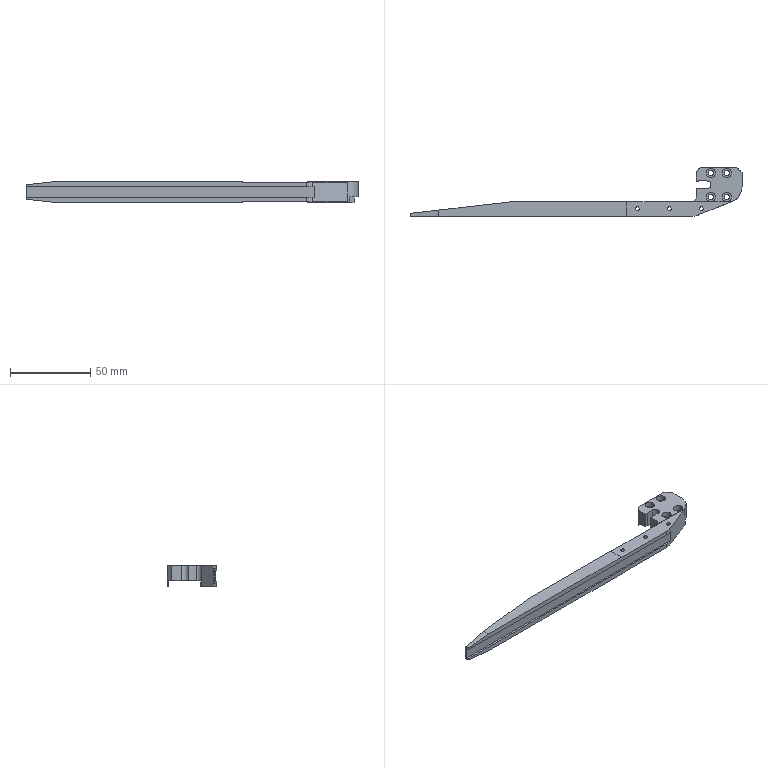NC program | NX | posted by the shop | part box 207.5 x 30.8 x 13 mm
Lines 86 to 1129 of 6162:
N5 T09 M06
(D10  D=10. R=0. H=09 ce=0.10 di=0.10)
G00 G90 G54 X-59. Y29.9 M03 S8000
G43 H09 Z10.2
M08
Z1.
G01 Z-.2 F4000.
Y25.4
G03 X-52. Y18.4 I7. J0.0
G01 X106.25
G02 X106.75 Y17.9 I0.0 J-.5
G01 Y-17.9
G02 X106.25 Y-18.4 I-.5 J0.0
G01 X94.013
G02 X89.053 Y-21.772 I-5.655 J2.985
G01 X88.423 Y-21.839
X87.44 Y-21.9
X-31.75
G02 X-37.516 Y-18.4 I0.0 J6.5
G01 X-106.25
G02 X-106.75 Y-17.9 I0.0 J.5
G01 Y10.936
G02 X-107.75 Y14.4 I5.5 J3.464
X-106.75 Y17.864 I6.5 J0.0
G01 Y17.9
G02 X-106.389 Y18.38 I.5 J0.0
X-105.846 Y18.996 I5.139 J-3.98
G01 X-104.846 Y19.996
G02 X-100.25 Y21.9 I4.596 J-4.596
G01 X-77.646 Y21.899
G02 X-74.946 Y21.264 I-.064 J-6.329
X-73.178 Y20.02 I-2.804 J-5.864
X-72.132 Y18.974 I-9.381 J-10.427
X-71.627 Y18.4 I-4.618 J-4.574
G01 X-50.014
G02 X-49.201 Y17.982 I0.0 J-1.
G01 X-44.799 Y11.818
G03 X-43.986 Y11.4 I.813 J.582
G01 X65.138
G02 X65.928 Y11.012 I-.001 J-1.
G01 X69.76 Y6.052
X69.771 Y6.039
G02 X70.319 Y4.477 I-1.952 J-1.562
X67.819 Y1.977 I-2.5 J0.0
G01 X67.797
X-39.455 Y2.88
G02 X-41.934 Y5.38 I.021 J2.5
X-39.434 Y7.88 I2.5 J0.0
G01 X-39.412
X65.211 Y6.999
X65.219
G03 X65.924 Y7.29 I0.0 J1.
G01 X69.758 Y11.109
G02 X70.464 Y11.4 I.706 J-.709
G01 X98.754
G02 X99.75 Y10.404 I-.004 J-1.
G01 Y-10.404
G02 X98.754 Y-11.4 I-1. J.004
G01 X95.648
G02 X94.666 Y-10.569 I.004 J1.
G03 X91.848 Y-6.298 I-6.221 J-1.04
X88.501 Y-5.12 I-4.175 J-6.517
G01 X87.728 Y-5.015
X72.969 Y-3.319
G02 X72.11 Y-2.552 I.115 J.993
G01 X70.666 Y3.654
G03 X70.457 Y4.071 I-.974 J-.227
G01 X70.41 Y4.2
G02 X70.608 Y4.4 I.2 J0.0
G01 X91.754
G02 X92.75 Y3.404 I-.004 J-1.
G01 Y2.383
G02 X91.75 Y1.387 I-1. J.004
X91.495 Y1.42 I0.0 J1.
G03 X89.363 Y1.827 I-3.822 J-14.236
G01 X88.564 Y1.935
X73.58 Y3.657
X73.466 Y3.664
G03 X72.724 Y3.334 I0.0 J-1.
G01 X67.647 Y-2.286
G02 X66.905 Y-2.615 I-.742 J.671
G01 X66.791 Y-2.608
X40.992 Y.357
G03 X40.25 Y.4 I-.742 J-6.457
G01 X-31.75
G03 X-38.25 Y-6.1 I0.0 J-6.5
G01 Y-9.911
G03 X-37.805 Y-10.615 I.779 J0.0
G01 X-37.45 Y-10.783
X-37.27 Y-10.824
G03 X-36.85 Y-10.404 I0.0 J.42
G01 Y-6.1
G02 X-31.75 Y-1. I5.1 J0.0
G01 X40.25
G02 X40.832 Y-1.033 I0.0 J-5.1
G01 X63.867 Y-3.681
X78.573 Y-5.372
X87.568 Y-6.406
X88.332 Y-6.51
G02 X91.093 Y-7.477 I-.66 J-6.306
X93.353 Y-11.609 I-2.647 J-4.132
G01 Y-15.415
G02 X88.901 Y-20.38 I-4.995 J0.0
G01 X88.332 Y-20.442
X87.44 Y-20.5
X-31.75
G02 X-36.85 Y-15.4 I0.0 J5.1
G01 Y-10.404
G03 X-37.27 Y-9.984 I-.42 J0.0
G01 X-37.45 Y-10.024
X-38.048 Y-10.308
G03 X-38.269 Y-10.592 I.172 J-.361
G02 X-39.246 Y-11.4 I-.981 J.192
G01 X-66.109
G02 X-67.105 Y-10.4 I.004 J1.
X-66.926 Y-9.829 I1. J0.0
G03 X-65.75 Y-6.1 I-5.324 J3.729
X-71.108 Y.299 I-6.5 J0.0
G02 X-71.323 Y.364 I.179 J.984
G03 X-73.908 Y.9 I-2.585 J-5.964
G01 X-98.17
X-98.195
G03 X-98.838 Y.455 I.003 J-.692
G01 X-98.992 Y.053
X-99.02 Y-.097
G03 X-98.6 Y-.517 I.42 J0.0
G01 X-98.567 Y-.515
G02 X-98.17 Y-.5 I.397 J-5.084
G01 X-73.908
G02 X-71.628 Y-1.038 I0.0 J-5.1
X-67.15 Y-6.1 I-.622 J-5.062
X-72.25 Y-11.2 I-5.1 J0.0
G01 X-97.
G02 X-98.894 Y-10.835 I0.0 J5.1
X-99.245 Y-10.695 I2.083 J5.717
G01 X-99.358 Y-10.65
G02 X-100.425 Y-10.174 I5.608 J14.02
X-103.27 Y-5.6 I2.255 J4.574
X-98.567 Y-.515 I5.1 J0.0
G03 X-98.18 Y-.097 I-.033 J.419
X-98.235 Y.112 I-.42 J0.0
G01 X-98.565 Y.686
G03 X-98.865 Y.884 I-.347 J-.199
G02 X-99.75 Y1.874 I.115 J.993
G01 Y6.904
G02 X-98.754 Y7.9 I1. J-.004
G01 X-76.745
G03 X-74.364 Y8.352 I0.0 J6.489
G02 X-73.997 Y8.422 I.367 J-.93
X-73.631 Y8.353 I0.0 J-1.
G01 X-71.837 Y7.648
G03 X-71.471 Y7.579 I.366 J.931
G01 X-71.408 Y7.581
X-64.731 Y8.008
X-64.571 Y8.014
G02 X-62.071 Y5.514 I0.0 J-2.5
X-64.411 Y3.019 I-2.5 J0.0
G01 X-72.12 Y2.525
X-72.28 Y2.52
G02 X-74.78 Y5.02 I0.0 J2.5
X-73.04 Y7.401 I2.5 J0.0
G03 X-72.352 Y8.232 I-.304 J.953
G01 X-72.183 Y9.608
G02 X-72.069 Y9.964 I.993 J-.122
G01 X-71.449 Y11.105
G03 X-71.379 Y11.378 I-.502 J.273
X-71.951 Y11.949 I-.572 J0.0
X-72.434 Y11.682 I0.0 J-.572
G02 X-72.763 Y11.22 I-4.316 J2.718
X-76.745 Y9.3 I-3.982 J3.169
G01 X-101.25
G02 X-106.35 Y14.4 I0.0 J5.1
X-104.856 Y18.006 I5.1 J0.0
G01 X-103.856 Y19.006
G02 X-100.25 Y20.5 I3.606 J-3.606
G01 X-77.665 Y20.499
G02 X-75.554 Y20.003 I-.046 J-4.929
X-74.14 Y19.002 I-2.196 J-4.603
X-73.144 Y18.006 I-8.416 J-9.412
X-71.65 Y14.4 I-3.606 J-3.606
X-72.434 Y11.682 I-5.1 J0.0
G03 X-72.499 Y11.458 I.355 J-.224
X-72.129 Y11.041 I.42 J0.0
G01 X-71.472 Y10.963
X-71.425 Y10.96
G03 X-71.134 Y11.086 I0.0 J.4
G02 X-70.409 Y11.4 I.728 J-.686
G01 X-50.014
G02 X-49.201 Y10.982 I0.0 J-1.
G01 X-44.799 Y4.819
G03 X-43.986 Y4.4 I.814 J.582
G01 X-42.7
G02 X-41.704 Y3.4 I-.004 J-1.
X-41.946 Y2.748 I-1. J0.0
G03 X-45.015 Y-3.59 I10.196 J-8.848
G02 X-45.992 Y-4.4 I-.982 J.19
G01 X-58.008
G02 X-58.985 Y-3.59 I.004 J1.
G03 X-62.054 Y2.748 I-13.265 J-2.51
G02 X-62.296 Y3.4 I.758 J.652
X-61.3 Y4.4 I1. J0.0
G01 X-47.
X-46.5
G03 X-39.5 Y11.4 I0.0 J7.
G01 Y29.9
Z1.
G00 Z3.
G01 X74.181 F6000.
G00 Z.38
G01 Z-.82 F4000.
Y25.4
G03 X81.181 Y18.4 I7. J0.0
G01 X106.25
G02 X106.75 Y17.9 I0.0 J-.5
G01 Y-17.9
G02 X106.25 Y-18.4 I-.5 J0.0
G01 X99.662
G02 X94.394 Y-21.809 I-5.659 J2.971
G01 X92.863 Y-21.9
X-71.824
G02 X-77.952 Y-20.72 I0.0 J16.5
G01 X-83.752 Y-18.4
X-106.25
G02 X-106.75 Y-17.9 I0.0 J.5
G01 Y10.936
G02 X-107.75 Y14.4 I5.5 J3.464
X-106.75 Y17.864 I6.5 J0.0
G01 Y17.9
G02 X-106.389 Y18.38 I.5 J0.0
X-105.846 Y18.996 I5.139 J-3.98
G01 X-104.846 Y19.996
G02 X-100.25 Y21.9 I4.596 J-4.596
G01 X-77.646 Y21.899
G02 X-74.946 Y21.264 I-.064 J-6.329
X-73.178 Y20.02 I-2.804 J-5.864
X-72.132 Y18.974 I-9.381 J-10.427
X-71.627 Y18.4 I-4.618 J-4.574
G01 X86.181
G02 X87.152 Y17.638 I0.0 J-1.
G01 X88.495 Y12.162
G03 X89.465 Y11.4 I.971 J.238
G01 X98.754
G02 X99.75 Y10.404 I-.004 J-1.
G01 Y-6.588
G02 X98.75 Y-7.584 I-1. J.004
X98.109 Y-7.352 I0.0 J1.
G03 X95.162 Y-5.954 I-4.133 J-4.91
G01 X94.048 Y-5.747
X93.836 Y-5.717
X40.992 Y.357
G03 X40.25 Y.4 I-.742 J-6.457
G01 X-71.219
G02 X-71.571 Y.465 I.004 J1.
G03 X-73.908 Y.9 I-2.337 J-6.065
G01 X-98.17
X-98.195
G03 X-98.839 Y.455 I.003 J-.692
G01 X-98.992 Y.053
X-99.02 Y-.097
G03 X-98.6 Y-.517 I.42 J0.0
G01 X-98.567 Y-.515
G02 X-98.17 Y-.5 I.397 J-5.084
G01 X-73.908
G02 X-71.706 Y-1. I0.0 J-5.1
G01 X40.25
G02 X40.832 Y-1.033 I0.0 J-5.1
G01 X63.867 Y-3.681
X65.145 Y-3.828
X78.573 Y-5.372
X81.531 Y-5.712
X93.676 Y-7.108
X93.854 Y-7.133
X94.903 Y-7.33
G02 X98.994 Y-12.262 I-.927 J-4.932
G01 Y-15.429
G02 X94.308 Y-20.411 I-4.992 J0.0
G01 X92.863 Y-20.5
X-71.824
G02 X-77.432 Y-19.42 I0.0 J15.1
G01 X-98.894 Y-10.835
G02 X-99.245 Y-10.695 I2.083 J5.717
G01 X-99.357 Y-10.65
G02 X-100.425 Y-10.174 I5.607 J14.02
X-103.27 Y-5.6 I2.255 J4.574
X-98.567 Y-.515 I5.1 J0.0
G03 X-98.18 Y-.097 I-.033 J.419
X-98.236 Y.112 I-.42 J0.0
G01 X-98.565 Y.686
G03 X-98.865 Y.884 I-.347 J-.199
G02 X-99.75 Y1.874 I.115 J.993
G01 Y6.904
G02 X-98.754 Y7.9 I1. J-.004
G01 X-76.745
G03 X-74.512 Y8.296 I0.0 J6.489
G02 X-74.217 Y8.349 I.295 J-.804
X-73.932 Y8.3 I0.0 J-.856
G01 X-72.879 Y7.928
G03 X-72.547 Y7.871 I.332 J.943
G01 X-72.389 Y7.884
G02 X-71.99 Y7.916 I.399 J-2.468
G01 X-71.973
X67.835 Y6.981
G02 X70.319 Y4.481 I-.017 J-2.5
X67.819 Y1.981 I-2.5 J0.0
G01 X67.802
X-72.006 Y2.916
G02 X-74.49 Y5.416 I.017 J2.5
X-73.396 Y7.483 I2.5 J0.0
G03 X-73.035 Y7.926 I-.563 J.826
G01 X-72.355 Y9.569
X-72.292 Y9.695
X-71.467 Y11.092
G03 X-71.388 Y11.38 I-.488 J.288
X-71.955 Y11.947 I-.567 J0.0
X-72.434 Y11.682 I0.0 J-.567
G02 X-72.763 Y11.22 I-4.316 J2.718
X-76.745 Y9.3 I-3.982 J3.169
G01 X-76.75
X-101.25
G02 X-106.35 Y14.4 I0.0 J5.1
X-104.856 Y18.006 I5.1 J0.0
G01 X-103.856 Y19.006
G02 X-100.25 Y20.5 I3.606 J-3.606
G01 X-77.665 Y20.499
G02 X-75.554 Y20.003 I-.046 J-4.929
X-74.14 Y19.002 I-2.196 J-4.603
X-73.144 Y18.006 I-8.416 J-9.412
X-71.65 Y14.4 I-3.606 J-3.606
X-72.434 Y11.682 I-5.1 J0.0
G03 X-72.499 Y11.459 I.355 J-.224
X-72.129 Y11.041 I.42 J0.0
G01 X-71.472 Y10.963
X-71.425 Y10.96
G03 X-71.134 Y11.085 I0.0 J.4
G02 X-70.409 Y11.4 I.728 J-.685
G01 X83.167
G02 X83.98 Y10.982 I-.001 J-1.
G01 X88.382 Y4.819
G03 X89.196 Y4.4 I.814 J.581
G01 X91.754
G02 X92.75 Y3.404 I-.004 J-1.
G01 Y2.571
G02 X91.75 Y1.575 I-1. J.004
G01 X91.64 Y1.581
X70.585 Y4.002
G02 X70.41 Y4.2 I.025 J.198
X70.608 Y4.4 I.2 J0.0
G01 X86.181
X86.681
G03 X93.681 Y11.4 I0.0 J7.
G01 Y29.9
Z.38
G00 Z2.8
G01 X74.181 F6000.
G00 Z-.24
G01 Z-1.44 F4000.
Y25.4
G03 X81.181 Y18.4 I7. J0.0
G01 X106.25
G02 X106.75 Y17.9 I0.0 J-.5
G01 Y-17.9
G02 X106.25 Y-18.4 I-.5 J0.0
G01 X105.201
G02 X100.684 Y-21.704 I-5.659 J2.998
X98.486 Y-21.901 I-2.198 J12.128
G01 X98.318 Y-21.9
X-71.824
G02 X-77.952 Y-20.72 I0.0 J16.5
G01 X-83.752 Y-18.4
X-106.25
G02 X-106.75 Y-17.9 I0.0 J.5
G01 Y10.936
G02 X-107.75 Y14.4 I5.5 J3.464
X-106.75 Y17.864 I6.5 J0.0
G01 Y17.9
G02 X-106.389 Y18.38 I.5 J0.0
X-105.846 Y18.996 I5.139 J-3.98
G01 X-104.846 Y19.996
G02 X-100.25 Y21.9 I4.596 J-4.596
G01 X-77.646 Y21.899
G02 X-74.946 Y21.264 I-.064 J-6.329
X-73.178 Y20.02 I-2.804 J-5.864
X-72.132 Y18.974 I-9.381 J-10.427
X-71.627 Y18.4 I-4.618 J-4.574
G01 X86.181
G02 X87.153 Y17.638 I0.0 J-1.
G01 X88.495 Y12.162
G03 X89.465 Y11.4 I.971 J.238
G01 X98.754
G02 X99.75 Y10.404 I-.004 J-1.
G01 Y-5.28
G02 X98.75 Y-6.276 I-1. J.004
G01 X98.64 Y-6.27
X40.992 Y.357
G03 X40.25 Y.4 I-.742 J-6.457
G01 X-71.22
G02 X-71.571 Y.465 I.004 J1.
G03 X-73.908 Y.9 I-2.337 J-6.065
G01 X-98.17
X-98.195
G03 X-98.839 Y.455 I.003 J-.692
G01 X-98.992 Y.053
X-99.02 Y-.097
G03 X-98.6 Y-.517 I.42 J0.0
G01 X-98.567 Y-.515
G02 X-98.17 Y-.5 I.397 J-5.084
G01 X-73.908
G02 X-71.706 Y-1. I0.0 J-5.1
G01 X40.25
G02 X40.832 Y-1.033 I0.0 J-5.1
G01 X78.573 Y-5.372
X81.531 Y-5.712
X93.676 Y-7.108
X99.142 Y-7.737
X100.347 Y-7.941
G02 X104.547 Y-12.913 I-.843 J-4.972
G01 Y-15.402
G02 X100.435 Y-20.326 I-5.004 J0.0
X98.486 Y-20.501 I-1.949 J10.751
G01 X98.327 Y-20.5
X-71.824
G02 X-77.432 Y-19.42 I0.0 J15.1
G01 X-98.894 Y-10.835
G02 X-99.245 Y-10.695 I2.083 J5.717
G01 X-99.356 Y-10.65
G02 X-100.427 Y-10.173 I5.606 J14.021
X-103.27 Y-5.6 I2.257 J4.573
X-98.567 Y-.515 I5.1 J0.0
G03 X-98.18 Y-.097 I-.033 J.419
X-98.236 Y.112 I-.42 J0.0
G01 X-98.565 Y.686
G03 X-98.866 Y.884 I-.347 J-.199
G02 X-99.75 Y1.873 I.115 J.993
G01 Y6.904
G02 X-98.754 Y7.9 I1. J-.004
G01 X-76.745
G03 X-74.512 Y8.296 I0.0 J6.489
G02 X-74.217 Y8.349 I.295 J-.804
X-73.932 Y8.3 I0.0 J-.856
G01 X-72.879 Y7.928
G03 X-72.547 Y7.871 I.332 J.943
G01 X-72.389 Y7.884
G02 X-71.99 Y7.916 I.399 J-2.468
G01 X-71.973
X67.835 Y6.981
G02 X70.319 Y4.481 I-.017 J-2.5
X67.819 Y1.981 I-2.5 J0.0
G01 X67.802
X-72.006 Y2.916
G02 X-74.49 Y5.416 I.017 J2.5
X-73.396 Y7.483 I2.5 J0.0
G03 X-73.035 Y7.926 I-.563 J.826
G01 X-72.355 Y9.57
X-72.292 Y9.696
X-71.467 Y11.092
G03 X-71.388 Y11.38 I-.488 J.288
X-71.955 Y11.947 I-.567 J0.0
X-72.434 Y11.682 I0.0 J-.567
G02 X-72.763 Y11.22 I-4.316 J2.718
X-76.745 Y9.3 I-3.982 J3.169
G01 X-76.75
X-101.25
G02 X-106.35 Y14.4 I0.0 J5.1
X-104.856 Y18.006 I5.1 J0.0
G01 X-103.856 Y19.006
G02 X-100.25 Y20.5 I3.606 J-3.606
G01 X-77.665 Y20.499
G02 X-75.554 Y20.003 I-.046 J-4.929
X-74.14 Y19.002 I-2.196 J-4.603
X-73.144 Y18.006 I-8.416 J-9.412
X-71.65 Y14.4 I-3.606 J-3.606
X-72.434 Y11.682 I-5.1 J0.0
G03 X-72.499 Y11.459 I.355 J-.224
X-72.129 Y11.042 I.42 J0.0
G01 X-71.471 Y10.963
X-71.424 Y10.96
G03 X-71.134 Y11.086 I0.0 J.4
G02 X-70.41 Y11.4 I.728 J-.686
G01 X83.168
G02 X83.98 Y10.982 I-.001 J-1.
G01 X88.382 Y4.819
G03 X89.196 Y4.4 I.814 J.581
G01 X91.755
G02 X92.75 Y3.405 I-.004 J-1.
G01 Y2.571
G02 X91.75 Y1.575 I-1. J.004
G01 X91.64 Y1.581
X70.585 Y4.002
G02 X70.41 Y4.2 I.025 J.198
X70.608 Y4.4 I.2 J0.0
G01 X86.181
X86.681
G03 X93.681 Y11.4 I0.0 J7.
G01 Y29.9
Z-.24
G00 Z2.18
G01 X74.181 F6000.
G00 Z-.86
G01 Z-2.06 F4000.
Y25.4
G03 X81.181 Y18.4 I7. J0.0
G01 X106.25
G02 X106.75 Y17.9 I0.0 J-.5
G01 Y-7.784
G02 X110.25 Y-13.846 I-3.5 J-6.062
G01 Y-14.4
G02 X102.75 Y-21.9 I-7.5 J0.0
G01 X-71.824
G02 X-77.952 Y-20.72 I0.0 J16.5
G01 X-83.752 Y-18.4
X-106.25
G02 X-106.75 Y-17.9 I0.0 J.5
G01 Y10.936
G02 X-107.75 Y14.4 I5.5 J3.464
X-106.75 Y17.864 I6.5 J0.0
G01 Y17.9
G02 X-106.389 Y18.38 I.5 J0.0
X-105.846 Y18.996 I5.139 J-3.98
G01 X-104.846 Y19.996
G02 X-100.25 Y21.9 I4.596 J-4.596
G01 X-77.646 Y21.899
G02 X-74.946 Y21.264 I-.064 J-6.329
X-73.178 Y20.02 I-2.804 J-5.864
X-72.132 Y18.974 I-9.381 J-10.427
X-71.627 Y18.4 I-4.618 J-4.574
G01 X86.181
G02 X87.153 Y17.638 I0.0 J-1.
G01 X88.495 Y12.162
G03 X89.466 Y11.4 I.971 J.238
G01 X98.754
G02 X99.75 Y10.404 I-.004 J-1.
G01 Y-5.28
G02 X98.75 Y-6.276 I-1. J.004
G01 X98.64 Y-6.27
X40.992 Y.357
G03 X40.25 Y.4 I-.742 J-6.457
G01 X-71.22
G02 X-71.571 Y.465 I.004 J1.
G03 X-73.908 Y.9 I-2.337 J-6.065
G01 X-98.171
X-98.195
G03 X-98.839 Y.455 I.003 J-.692
G01 X-98.993 Y.053
X-99.02 Y-.097
G03 X-98.6 Y-.517 I.42 J0.0
G01 X-98.568 Y-.516
G02 X-98.17 Y-.5 I.398 J-5.084
G01 X-98.16
X-73.908
G02 X-71.706 Y-1. I0.0 J-5.1
G01 X40.25
G02 X40.832 Y-1.033 I0.0 J-5.1
G01 X81.09 Y-5.661
X81.531 Y-5.712
X83.818 Y-5.975
X103.89 Y-8.282
G02 X108.85 Y-13.846 I-.64 J-5.563
G01 Y-14.4
G02 X102.75 Y-20.5 I-6.1 J0.0
G01 X-71.824
G02 X-77.432 Y-19.42 I0.0 J15.1
G01 X-98.894 Y-10.835
G02 X-99.245 Y-10.695 I2.083 J5.717
G01 X-99.355 Y-10.651
G02 X-100.428 Y-10.173 I5.605 J14.021
X-103.27 Y-5.6 I2.258 J4.573
X-98.568 Y-.516 I5.1 J0.0
G03 X-98.18 Y-.097 I-.033 J.419
X-98.236 Y.112 I-.42 J0.0
G01 X-98.565 Y.686
G03 X-98.866 Y.884 I-.347 J-.199
G02 X-99.75 Y1.873 I.116 J.993
G01 Y6.904
G02 X-98.754 Y7.9 I1. J-.004
G01 X-76.745
G03 X-74.512 Y8.296 I0.0 J6.489
G02 X-74.217 Y8.349 I.295 J-.804
X-73.932 Y8.3 I0.0 J-.856
G01 X-72.879 Y7.928
G03 X-72.547 Y7.871 I.332 J.943
G01 X-72.389 Y7.884
G02 X-71.99 Y7.916 I.399 J-2.468
G01 X-71.973
X67.835 Y6.981
G02 X70.318 Y4.481 I-.017 J-2.5
X67.818 Y1.981 I-2.5 J0.0
G01 X67.802
X-72.006 Y2.916
G02 X-74.49 Y5.416 I.017 J2.5
X-73.396 Y7.483 I2.5 J0.0
G03 X-73.035 Y7.926 I-.563 J.826
G01 X-72.355 Y9.57
X-72.292 Y9.696
X-71.467 Y11.092
G03 X-71.388 Y11.381 I-.488 J.288
X-71.955 Y11.948 I-.567 J0.0
X-72.434 Y11.683 I0.0 J-.567
G02 X-72.763 Y11.22 I-4.316 J2.717
X-76.745 Y9.3 I-3.982 J3.169
G01 X-76.75
X-101.25
G02 X-106.35 Y14.4 I0.0 J5.1
X-104.856 Y18.006 I5.1 J0.0
G01 X-103.856 Y19.006
G02 X-100.25 Y20.5 I3.606 J-3.606
G01 X-77.665 Y20.499
G02 X-75.554 Y20.003 I-.046 J-4.929
X-74.14 Y19.002 I-2.196 J-4.603
X-73.144 Y18.006 I-8.416 J-9.412
X-71.65 Y14.4 I-3.606 J-3.606
X-72.434 Y11.683 I-5.1 J0.0
G03 X-72.499 Y11.459 I.355 J-.224
X-72.129 Y11.042 I.42 J0.0
G01 X-71.471 Y10.963
X-71.424 Y10.961
G03 X-71.134 Y11.086 I0.0 J.4
G02 X-70.41 Y11.4 I.728 J-.686
G01 X83.168
G02 X83.98 Y10.982 I-.001 J-1.
G01 X88.382 Y4.819
G03 X89.196 Y4.4 I.814 J.581
G01 X91.755
G02 X92.75 Y3.405 I-.005 J-1.
G01 Y2.57
G02 X91.75 Y1.575 I-1. J.005
G01 X91.641 Y1.581
X70.585 Y4.002
G02 X70.41 Y4.2 I.025 J.198
X70.608 Y4.4 I.2 J0.0
G01 X86.181
X86.681
G03 X93.681 Y11.4 I0.0 J7.
G01 Y29.9
Z-.86
G00 Z1.56
G01 X74.181 F6000.
G00 Z-1.48
G01 Z-2.68 F4000.
Y25.4
G03 X81.181 Y18.4 I7. J0.0
G01 X106.25
G02 X106.75 Y17.9 I0.0 J-.5
G01 Y-7.784
G02 X110.25 Y-13.846 I-3.5 J-6.062
G01 Y-14.4
G02 X102.75 Y-21.9 I-7.5 J0.0
G01 X-71.824
G02 X-77.952 Y-20.72 I0.0 J16.5
G01 X-83.752 Y-18.4
X-106.25
G02 X-106.75 Y-17.9 I0.0 J.5
G01 Y10.936
G02 X-107.75 Y14.4 I5.5 J3.464
X-106.75 Y17.864 I6.5 J0.0
G01 Y17.9
G02 X-106.389 Y18.38 I.5 J0.0
X-105.846 Y18.996 I5.139 J-3.98
G01 X-104.846 Y19.996
G02 X-100.25 Y21.9 I4.596 J-4.596
G01 X-77.646 Y21.899
G02 X-74.946 Y21.264 I-.064 J-6.329
X-73.178 Y20.02 I-2.804 J-5.864
X-72.132 Y18.974 I-9.381 J-10.427
X-71.627 Y18.4 I-4.618 J-4.574
G01 X86.181
G02 X87.153 Y17.638 I0.0 J-1.
G01 X88.495 Y12.162
G03 X89.466 Y11.4 I.971 J.238
G01 X98.755
G02 X99.75 Y10.405 I-.005 J-1.
G01 Y-5.28
G02 X98.75 Y-6.276 I-1. J.005
G01 X98.64 Y-6.27
X40.992 Y.357
G03 X40.25 Y.4 I-.742 J-6.457
G01 X-71.22
G02 X-71.571 Y.465 I.005 J1.
G03 X-73.908 Y.9 I-2.338 J-6.065
G01 X-98.173
X-98.196
G03 X-98.839 Y.455 I.003 J-.692
G01 X-98.993 Y.053
X-99.02 Y-.097
G03 X-98.6 Y-.517 I.42 J0.0
G01 X-98.568 Y-.516
G02 X-98.17 Y-.5 I.398 J-5.084
G01 X-98.16
X-73.908
G02 X-71.706 Y-1. I0.0 J-5.1
G01 X40.25
G02 X40.832 Y-1.033 I0.0 J-5.1
G01 X103.89 Y-8.282
G02 X108.85 Y-13.846 I-.64 J-5.563
G01 Y-14.4
G02 X102.75 Y-20.5 I-6.1 J0.0
G01 X-71.824
G02 X-77.432 Y-19.42 I0.0 J15.1
G01 X-98.894 Y-10.835
G02 X-99.245 Y-10.695 I2.083 J5.717
G01 X-99.355 Y-10.651
G02 X-100.43 Y-10.172 I5.605 J14.021
X-103.27 Y-5.6 I2.26 J4.572
X-98.568 Y-.516 I5.1 J0.0
G03 X-98.18 Y-.097 I-.033 J.419
X-98.236 Y.112 I-.42 J0.0
G01 X-98.566 Y.686
G03 X-98.866 Y.884 I-.347 J-.199
G02 X-99.75 Y1.873 I.116 J.993
G01 Y6.905
G02 X-98.755 Y7.9 I1. J-.005
G01 X-76.745
G03 X-74.512 Y8.296 I0.0 J6.489
G02 X-74.217 Y8.349 I.295 J-.804
X-73.932 Y8.3 I0.0 J-.856
G01 X-72.879 Y7.928
G03 X-72.547 Y7.871 I.332 J.943
G01 X-72.389 Y7.884
G02 X-71.99 Y7.916 I.399 J-2.468
G01 X-71.973
X67.835 Y6.981
G02 X70.318 Y4.481 I-.017 J-2.5
X67.818 Y1.981 I-2.5 J0.0
G01 X67.802
X-72.006 Y2.916
G02 X-74.49 Y5.416 I.017 J2.5
X-73.396 Y7.483 I2.5 J0.0
G03 X-73.035 Y7.926 I-.563 J.826
G01 X-72.355 Y9.57
X-72.292 Y9.696
X-71.467 Y11.092
G03 X-71.388 Y11.381 I-.488 J.288
X-71.954 Y11.948 I-.567 J0.0
X-72.434 Y11.683 I0.0 J-.567
G02 X-72.763 Y11.22 I-4.316 J2.717
X-76.745 Y9.3 I-3.982 J3.169
G01 X-76.75
X-101.25
G02 X-106.35 Y14.4 I0.0 J5.1
X-104.856 Y18.006 I5.1 J0.0
G01 X-103.856 Y19.006
G02 X-100.25 Y20.5 I3.606 J-3.606
G01 X-77.664 Y20.499
G02 X-75.554 Y20.003 I-.046 J-4.929
X-74.14 Y19.002 I-2.196 J-4.603
X-73.144 Y18.006 I-8.416 J-9.412
X-71.65 Y14.4 I-3.606 J-3.606
X-72.434 Y11.683 I-5.1 J0.0
G03 X-72.499 Y11.459 I.355 J-.224
X-72.129 Y11.042 I.42 J0.0
G01 X-71.471 Y10.963
X-71.424 Y10.961
G03 X-71.133 Y11.086 I0.0 J.4
G02 X-70.41 Y11.4 I.728 J-.686
G01 X83.168
G02 X83.98 Y10.982 I-.001 J-1.
G01 X88.382 Y4.819
G03 X89.196 Y4.4 I.814 J.581
G01 X91.755
G02 X92.75 Y3.405 I-.005 J-1.
G01 Y2.57
G02 X91.75 Y1.575 I-1. J.005
G01 X91.641 Y1.581
X70.585 Y4.002
G02 X70.41 Y4.2 I.025 J.198
X70.608 Y4.4 I.2 J0.0
G01 X86.181
X86.681
G03 X93.681 Y11.4 I0.0 J7.
G01 Y29.9
Z-1.48
G00 Z.94
G01 X74.181 F6000.
G00 Z-2.1
G01 Z-3.3 F4000.
Y25.4
G03 X81.181 Y18.4 I7. J0.0
G01 X106.25
G02 X106.75 Y17.9 I0.0 J-.5
G01 Y-7.784
G02 X110.25 Y-13.846 I-3.5 J-6.062
G01 Y-14.4
G02 X102.75 Y-21.9 I-7.5 J0.0
G01 X-71.824
G02 X-77.952 Y-20.72 I0.0 J16.5
G01 X-83.752 Y-18.4
X-106.25
G02 X-106.75 Y-17.9 I0.0 J.5
G01 Y10.936
G02 X-107.75 Y14.4 I5.5 J3.464
X-106.75 Y17.864 I6.5 J0.0
G01 Y17.9
G02 X-106.389 Y18.38 I.5 J0.0
X-105.846 Y18.996 I5.139 J-3.98
G01 X-104.846 Y19.996
G02 X-100.25 Y21.9 I4.596 J-4.596
G01 X-77.646 Y21.899
G02 X-74.946 Y21.264 I-.064 J-6.329
X-73.178 Y20.02 I-2.804 J-5.864
X-72.132 Y18.974 I-9.381 J-10.427
X-71.627 Y18.4 I-4.618 J-4.574
G01 X86.181
G02 X87.153 Y17.638 I0.0 J-1.
G01 X88.495 Y12.162
G03 X89.466 Y11.4 I.971 J.238
G01 X98.755
G02 X99.75 Y10.405 I-.005 J-1.
G01 Y-5.281
G02 X98.75 Y-6.276 I-1. J.005
G01 X98.641 Y-6.27
X40.992 Y.357
G03 X40.25 Y.4 I-.742 J-6.457
G01 X-71.22
G02 X-71.571 Y.465 I.005 J1.
G03 X-73.908 Y.9 I-2.338 J-6.065
G01 X-98.175
X-98.196
G03 X-98.84 Y.455 I.003 J-.692
G01 X-98.993 Y.053
X-99.021 Y-.097
G03 X-98.601 Y-.517 I.42 J0.0
G01 X-98.568 Y-.516
G02 X-98.17 Y-.5 I.398 J-5.084
G01 X-98.16
X-73.908
G02 X-71.706 Y-1. I0.0 J-5.1
G01 X40.25
G02 X40.832 Y-1.033 I0.0 J-5.1
G01 X103.89 Y-8.282
G02 X108.85 Y-13.846 I-.64 J-5.563
G01 Y-14.4
G02 X102.75 Y-20.5 I-6.1 J0.0
G01 X-71.824
G02 X-77.432 Y-19.42 I0.0 J15.1
G01 X-98.894 Y-10.835
G02 X-99.245 Y-10.695 I2.083 J5.717
G01 X-99.354 Y-10.651
G02 X-100.432 Y-10.171 I5.604 J14.021
X-103.27 Y-5.6 I2.261 J4.571
X-98.568 Y-.516 I5.1 J0.0
G03 X-98.181 Y-.097 I-.033 J.419
X-98.236 Y.112 I-.42 J0.0
G01 X-98.566 Y.686
G03 X-98.866 Y.884 I-.347 J-.199
G02 X-99.75 Y1.873 I.116 J.993
G01 Y6.905
G02 X-98.755 Y7.9 I1. J-.005
G01 X-76.745
G03 X-74.512 Y8.296 I0.0 J6.489
G02 X-74.217 Y8.349 I.295 J-.804
X-73.932 Y8.3 I0.0 J-.856
G01 X-72.879 Y7.928
G03 X-72.547 Y7.871 I.332 J.943
G01 X-72.389 Y7.884
G02 X-71.99 Y7.916 I.399 J-2.468
G01 X-71.973
X67.835 Y6.981
G02 X70.318 Y4.481 I-.017 J-2.5
X67.818 Y1.981 I-2.5 J0.0
G01 X67.802
X-72.006 Y2.916
G02 X-74.49 Y5.416 I.017 J2.5
X-73.396 Y7.483 I2.5 J0.0
G03 X-73.035 Y7.926 I-.563 J.826
G01 X-72.355 Y9.57
X-72.292 Y9.696
X-71.467 Y11.093
G03 X-71.388 Y11.381 I-.488 J.288
X-71.954 Y11.948 I-.567 J0.0
X-72.434 Y11.683 I0.0 J-.567
G02 X-72.763 Y11.22 I-4.316 J2.717
X-76.745 Y9.3 I-3.982 J3.169
G01 X-76.75
X-101.25
G02 X-106.35 Y14.4 I0.0 J5.1
X-104.856 Y18.006 I5.1 J0.0
G01 X-103.856 Y19.006
G02 X-100.25 Y20.5 I3.606 J-3.606
G01 X-77.664 Y20.499
G02 X-75.554 Y20.003 I-.046 J-4.929
X-74.14 Y19.002 I-2.196 J-4.603
X-73.144 Y18.006 I-8.416 J-9.412
X-71.65 Y14.4 I-3.606 J-3.606
X-72.434 Y11.683 I-5.1 J0.0
G03 X-72.499 Y11.459 I.355 J-.224
X-72.128 Y11.042 I.42 J0.0
G01 X-71.471 Y10.964
X-71.424 Y10.961
G03 X-71.133 Y11.086 I0.0 J.4
G02 X-70.41 Y11.4 I.728 J-.686
G01 X83.168
G02 X83.98 Y10.982 I-.001 J-1.
G01 X88.382 Y4.819
G03 X89.196 Y4.4 I.814 J.581
G01 X91.755
G02 X92.75 Y3.405 I-.005 J-1.
G01 Y2.57
G02 X91.75 Y1.575 I-1. J.005
G01 X91.641 Y1.581
X70.585 Y4.002
G02 X70.41 Y4.2 I.025 J.198
X70.608 Y4.4 I.2 J0.0
G01 X86.181
X86.681
G03 X93.681 Y11.4 I0.0 J7.
G01 Y29.9
Z-2.1
G00 Z.32
G01 X74.181 F6000.
G00 Z-2.59
G01 Z-3.79 F4000.
Y25.4
G03 X81.181 Y18.4 I7. J0.0
G01 X106.25
G02 X106.75 Y17.9 I0.0 J-.5
G01 Y-7.784
G02 X110.25 Y-13.846 I-3.5 J-6.062
G01 Y-14.4
G02 X102.75 Y-21.9 I-7.5 J0.0
G01 X-71.824
G02 X-77.952 Y-20.72 I0.0 J16.5
G01 X-83.752 Y-18.4
X-106.25
G02 X-106.75 Y-17.9 I0.0 J.5
G01 Y-6.791
G02 X-110.25 Y3.37 I13. J10.161
G01 Y11.9
G02 X-108.346 Y16.496 I6.5 J0.0
G01 X-106.668 Y18.174
G02 X-106.524 Y18.318 I.418 J-.274
G01 X-104.846 Y19.996
G02 X-100.25 Y21.9 I4.596 J-4.596
G01 X-77.646 Y21.899
G02 X-74.946 Y21.264 I-.064 J-6.329
X-73.178 Y20.02 I-2.804 J-5.864
X-72.133 Y18.975 I-9.381 J-10.427
G01 X-71.558 Y18.4
X86.181
G02 X87.153 Y17.638 I0.0 J-1.
G01 X88.495 Y12.162
G03 X89.466 Y11.4 I.971 J.238
G01 X98.755
G02 X99.75 Y10.405 I-.005 J-1.
G01 Y-5.281
G02 X98.75 Y-6.276 I-1. J.005
G01 X98.641 Y-6.27
X40.992 Y.357
G03 X40.25 Y.4 I-.742 J-6.457
G01 X-67.755
G02 X-68.75 Y1.395 I.005 J1.
G01 Y2.15
G03 X-69.051 Y4.104 I-6.5 J0.0
G02 X-69.095 Y4.4 I.955 J.296
X-69.051 Y4.696 I1. J0.0
G03 X-68.823 Y5.68 I-6.199 J1.954
G01 X-68.791 Y5.734
X-68.728 Y5.781
X-68.661 Y5.796
X-68.678 Y5.862
G02 X-66.218 Y7.917 I2.46 J-.445
G01 X-66.201
X67.836 Y6.981
G02 X70.318 Y4.481 I-.017 J-2.5
X67.818 Y1.981 I-2.5 J0.0
G01 X67.801
X-66.236 Y2.917
G02 X-68.718 Y5.417 I.017 J2.5
X-68.706 Y5.666 I2.5 J0.0
G01 X-68.722 Y5.724
X-68.77 Y5.785
X-68.83 Y5.82
X-68.796 Y5.881
G03 X-68.75 Y6.65 I-6.454 J.769
G01 Y9.913
G03 X-69.195 Y10.616 I-.779 J0.0
G01 X-69.55 Y10.784
X-69.73 Y10.825
G03 X-70.15 Y10.405 I0.0 J-.42
G01 Y6.65
G02 X-70.673 Y4.4 I-5.1 J0.0
X-70.15 Y2.15 I-4.577 J-2.25
G01 Y-1.
X40.25
G02 X40.832 Y-1.033 I0.0 J-5.1
G01 X103.89 Y-8.282
G02 X108.85 Y-13.846 I-.64 J-5.563
G01 Y-14.4
G02 X102.75 Y-20.5 I-6.1 J0.0
G01 X-71.824
G02 X-77.432 Y-19.42 I0.0 J15.1
G01 X-98.894 Y-10.835
G02 X-99.245 Y-10.695 I2.083 J5.717
G01 X-99.354 Y-10.651
G02 X-108.85 Y3.37 I5.604 J14.022
G01 Y11.9
G02 X-107.356 Y15.506 I5.1 J0.0
G01 X-103.856 Y19.006
G02 X-100.25 Y20.5 I3.606 J-3.606
G01 X-77.664 Y20.499
G02 X-75.554 Y20.003 I-.046 J-4.929
X-74.14 Y19.002 I-2.196 J-4.603
X-73.15 Y18.012 I-8.419 J-9.409
G01 X-71.644 Y16.506
G02 X-70.15 Y12.9 I-3.606 J-3.606
G01 Y10.405
G03 X-69.73 Y9.985 I.42 J0.0
G01 X-69.55 Y10.026
X-68.952 Y10.309
G03 X-68.731 Y10.593 I-.172 J.361
G02 X-67.755 Y11.4 I.981 J-.193
G01 X83.168
G02 X83.98 Y10.982 I-.001 J-1.
G01 X88.383 Y4.819
G03 X89.196 Y4.4 I.814 J.581
G01 X91.755
G02 X92.75 Y3.405 I-.005 J-1.
G01 Y2.57
G02 X91.75 Y1.575 I-1. J.005
G01 X91.641 Y1.581
X70.585 Y4.002
G02 X70.41 Y4.2 I.025 J.198
X70.608 Y4.4 I.2 J0.0
G01 X86.181
X86.681
G03 X93.681 Y11.4 I0.0 J7.
G01 Y29.9
Z-2.59
G00 Z-.3
G01 X74.182 F6000.
G00 Z-3.08
G01 Z-4.28 F4000.
Y25.4
G03 X81.182 Y18.4 I7. J0.0
G01 X106.25
G02 X106.75 Y17.9 I0.0 J-.5
G01 Y-7.784
G02 X110.25 Y-13.846 I-3.5 J-6.062
G01 Y-14.4
G02 X102.75 Y-21.9 I-7.5 J0.0
G01 X-71.824
G02 X-77.952 Y-20.72 I0.0 J16.5
G01 X-83.752 Y-18.4
X-106.25
G02 X-106.75 Y-17.9 I0.0 J.5
G01 Y-6.791